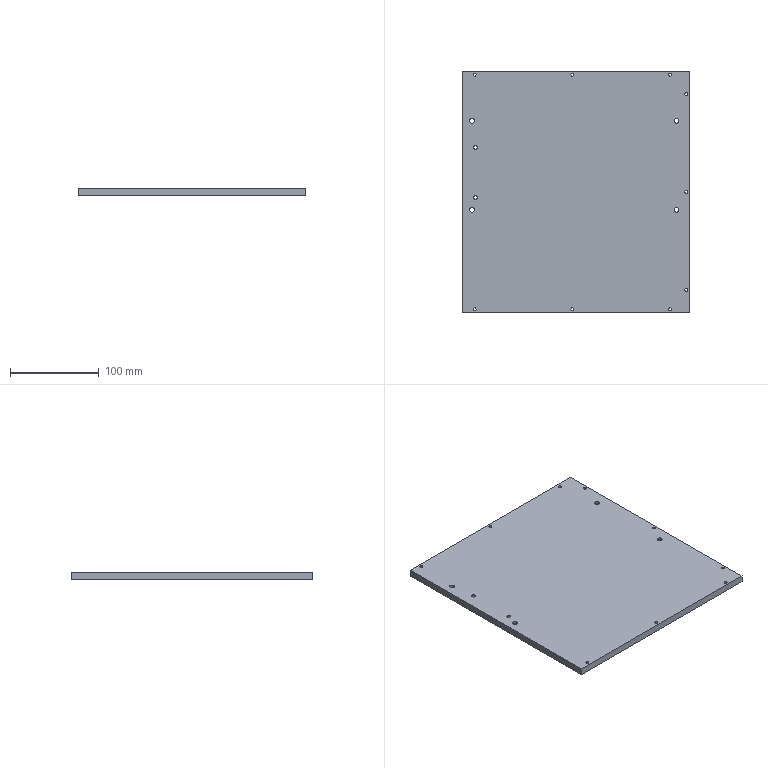Part | STEP file | CA-10-010Lift Stop Plate6_Default | 1 solid | 75 faces | box 256 x 272 x 8 mm | volume 553953 mm3 | cylinder 56 | plane 19 | commonest cylinder face diameters 5.5 x26 3.4 x18 9.5 x8 4.2 x4